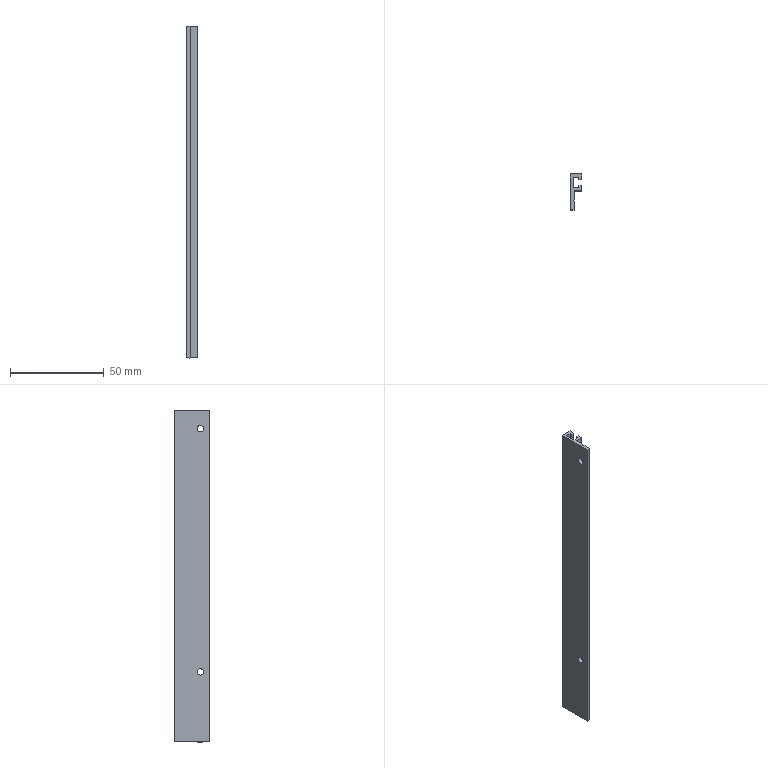Part | SolidWorks | features BaseBody 1 | 1 solid | 27 faces | box 6 x 19 x 177.5 mm | volume 9115 mm3 | plane 23 | cylinder 4 | commonest cylinder face diameters 3.4 x4
STEP:
#1=CARTESIAN_POINT('',(-62.496,1832.044,-25.2));
#2=VERTEX_POINT('',#1);
#3=CARTESIAN_POINT('',(-61.996,1831.544,-25.125));
#4=VERTEX_POINT('',#3);
#5=CARTESIAN_POINT('',(-62.496,1832.044,-25.2));
#6=CARTESIAN_POINT('',(-62.326,1831.874,-25.2));
#7=CARTESIAN_POINT('',(-62.158,1831.706,-25.175));
#8=CARTESIAN_POINT('',(-61.996,1831.544,-25.125));
#9=(BOUNDED_CURVE()B_SPLINE_CURVE(3,(#5,#6,#7,#8),.UNSPECIFIED.,.F.,.T.)B_SPLINE_CURVE_WITH_KNOTS((4,4),(1.571,1.869),.UNSPECIFIED.)CURVE()GEOMETRIC_REPRESENTATION_ITEM()RATIONAL_B_SPLINE_CURVE((1.,0.9926,0.9926,1.))REPRESENTATION_ITEM(''));
#10=EDGE_CURVE('',#2,#4,#9,.T.);
#11=ORIENTED_EDGE('',*,*,#10,.F.);
#12=CARTESIAN_POINT('',(-63.996,1832.044,-25.2));
#13=VERTEX_POINT('',#12);
#14=CARTESIAN_POINT('',(-63.996,1832.044,-25.2));
#15=DIRECTION('',(-1.,0.,0.));
#16=VECTOR('',#15,1000.);
#17=LINE('',#14,#16);
#18=EDGE_CURVE('',#2,#13,#17,.T.);
#19=ORIENTED_EDGE('',*,*,#18,.T.);
#20=CARTESIAN_POINT('',(-63.996,1832.044,-21.8));
#21=VERTEX_POINT('',#20);
#22=CARTESIAN_POINT('',(-63.996,1832.044,-23.5));
#23=DIRECTION('',(1.,0.,0.));
#24=DIRECTION('',(0.,0.,1.));
#25=AXIS2_PLACEMENT_3D('',#22,#23,#24);
#26=CIRCLE('',#25,1.7);
#27=EDGE_CURVE('',#21,#13,#26,.T.);
#28=ORIENTED_EDGE('',*,*,#27,.F.);
#29=CARTESIAN_POINT('',(-62.496,1832.044,-21.8));
#30=VERTEX_POINT('',#29);
#31=CARTESIAN_POINT('',(-63.996,1832.044,-21.8));
#32=DIRECTION('',(-1.,0.,0.));
#33=VECTOR('',#32,1000.);
#34=LINE('',#31,#33);
#35=EDGE_CURVE('',#30,#21,#34,.T.);
#36=ORIENTED_EDGE('',*,*,#35,.F.);
#37=CARTESIAN_POINT('',(-61.996,1831.544,-21.875));
#38=VERTEX_POINT('',#37);
#39=CARTESIAN_POINT('',(-61.996,1831.544,-21.875));
#40=CARTESIAN_POINT('',(-62.158,1831.706,-21.825));
#41=CARTESIAN_POINT('',(-62.326,1831.874,-21.8));
#42=CARTESIAN_POINT('',(-62.496,1832.044,-21.8));
#43=(BOUNDED_CURVE()B_SPLINE_CURVE(3,(#39,#40,#41,#42),.UNSPECIFIED.,.F.,.T.)B_SPLINE_CURVE_WITH_KNOTS((4,4),(4.414,4.712),.UNSPECIFIED.)CURVE()GEOMETRIC_REPRESENTATION_ITEM()RATIONAL_B_SPLINE_CURVE((1.,0.9926,0.9926,1.))REPRESENTATION_ITEM(''));
#44=EDGE_CURVE('',#38,#30,#43,.T.);
#45=ORIENTED_EDGE('',*,*,#44,.F.);
#46=CARTESIAN_POINT('',(-61.996,1832.044,-23.5));
#47=DIRECTION('',(-1.,0.,0.));
#48=DIRECTION('',(0.,0.,1.));
#49=AXIS2_PLACEMENT_3D('',#46,#47,#48);
#50=CIRCLE('',#49,1.7);
#51=EDGE_CURVE('',#4,#38,#50,.T.);
#52=ORIENTED_EDGE('',*,*,#51,.F.);
#53=EDGE_LOOP('',(#11,#19,#28,#36,#45,#52));
#54=FACE_OUTER_BOUND('',#53,.T.);
#55=CARTESIAN_POINT('',(-63.996,1832.044,-23.5));
#56=DIRECTION('',(-1.,0.,0.));
#57=DIRECTION('',(0.,0.,1.));
#58=AXIS2_PLACEMENT_3D('',#55,#56,#57);
#59=CYLINDRICAL_SURFACE('',#58,1.7);
#60=ADVANCED_FACE('',(#54),#59,.F.);
#61=CARTESIAN_POINT('',(-62.496,1832.044,-155.2));
#62=VERTEX_POINT('',#61);
#63=CARTESIAN_POINT('',(-61.996,1831.544,-155.125));
#64=VERTEX_POINT('',#63);
#65=CARTESIAN_POINT('',(-62.496,1832.044,-155.2));
#66=CARTESIAN_POINT('',(-62.326,1831.874,-155.2));
#67=CARTESIAN_POINT('',(-62.158,1831.706,-155.175));
#68=CARTESIAN_POINT('',(-61.996,1831.544,-155.125));
#69=(BOUNDED_CURVE()B_SPLINE_CURVE(3,(#65,#66,#67,#68),.UNSPECIFIED.,.F.,.T.)B_SPLINE_CURVE_WITH_KNOTS((4,4),(1.571,1.869),.UNSPECIFIED.)CURVE()GEOMETRIC_REPRESENTATION_ITEM()RATIONAL_B_SPLINE_CURVE((1.,0.9926,0.9926,1.))REPRESENTATION_ITEM(''));
#70=EDGE_CURVE('',#62,#64,#69,.T.);
#71=ORIENTED_EDGE('',*,*,#70,.F.);
#72=CARTESIAN_POINT('',(-63.996,1832.044,-155.2));
#73=VERTEX_POINT('',#72);
#74=CARTESIAN_POINT('',(-63.996,1832.044,-155.2));
#75=DIRECTION('',(-1.,0.,0.));
#76=VECTOR('',#75,1000.);
#77=LINE('',#74,#76);
#78=EDGE_CURVE('',#62,#73,#77,.T.);
#79=ORIENTED_EDGE('',*,*,#78,.T.);
#80=CARTESIAN_POINT('',(-63.996,1832.044,-151.8));
#81=VERTEX_POINT('',#80);
#82=CARTESIAN_POINT('',(-63.996,1832.044,-153.5));
#83=DIRECTION('',(1.,0.,0.));
#84=DIRECTION('',(0.,0.,1.));
#85=AXIS2_PLACEMENT_3D('',#82,#83,#84);
#86=CIRCLE('',#85,1.7);
#87=EDGE_CURVE('',#81,#73,#86,.T.);
#88=ORIENTED_EDGE('',*,*,#87,.F.);
#89=CARTESIAN_POINT('',(-62.496,1832.044,-151.8));
#90=VERTEX_POINT('',#89);
#91=CARTESIAN_POINT('',(-63.996,1832.044,-151.8));
#92=DIRECTION('',(-1.,0.,0.));
#93=VECTOR('',#92,1000.);
#94=LINE('',#91,#93);
#95=EDGE_CURVE('',#90,#81,#94,.T.);
#96=ORIENTED_EDGE('',*,*,#95,.F.);
#97=CARTESIAN_POINT('',(-61.996,1831.544,-151.875));
#98=VERTEX_POINT('',#97);
#99=CARTESIAN_POINT('',(-61.996,1831.544,-151.875));
#100=CARTESIAN_POINT('',(-62.158,1831.706,-151.825));
#101=CARTESIAN_POINT('',(-62.326,1831.874,-151.8));
#102=CARTESIAN_POINT('',(-62.496,1832.044,-151.8));
#103=(BOUNDED_CURVE()B_SPLINE_CURVE(3,(#99,#100,#101,#102),.UNSPECIFIED.,.F.,.T.)B_SPLINE_CURVE_WITH_KNOTS((4,4),(4.414,4.712),.UNSPECIFIED.)CURVE()GEOMETRIC_REPRESENTATION_ITEM()RATIONAL_B_SPLINE_CURVE((1.,0.9926,0.9926,1.))REPRESENTATION_ITEM(''));
#104=EDGE_CURVE('',#98,#90,#103,.T.);
#105=ORIENTED_EDGE('',*,*,#104,.F.);
#106=CARTESIAN_POINT('',(-61.996,1832.044,-153.5));
#107=DIRECTION('',(-1.,0.,0.));
#108=DIRECTION('',(0.,0.,1.));
#109=AXIS2_PLACEMENT_3D('',#106,#107,#108);
#110=CIRCLE('',#109,1.7);
#111=EDGE_CURVE('',#64,#98,#110,.T.);
#112=ORIENTED_EDGE('',*,*,#111,.F.);
#113=EDGE_LOOP('',(#71,#79,#88,#96,#105,#112));
#114=FACE_OUTER_BOUND('',#113,.T.);
#115=CARTESIAN_POINT('',(-63.996,1832.044,-153.5));
#116=DIRECTION('',(-1.,0.,0.));
#117=DIRECTION('',(0.,0.,1.));
#118=AXIS2_PLACEMENT_3D('',#115,#116,#117);
#119=CYLINDRICAL_SURFACE('',#118,1.7);
#120=ADVANCED_FACE('',(#114),#119,.F.);
#121=ORIENTED_EDGE('',*,*,#27,.T.);
#122=CARTESIAN_POINT('',(-63.996,1832.044,-23.5));
#123=DIRECTION('',(1.,0.,0.));
#124=DIRECTION('',(0.,0.,1.));
#125=AXIS2_PLACEMENT_3D('',#122,#123,#124);
#126=CIRCLE('',#125,1.7);
#127=EDGE_CURVE('',#13,#21,#126,.T.);
#128=ORIENTED_EDGE('',*,*,#127,.T.);
#129=EDGE_LOOP('',(#121,#128));
#130=FACE_BOUND('',#129,.T.);
#131=ORIENTED_EDGE('',*,*,#87,.T.);
#132=CARTESIAN_POINT('',(-63.996,1832.044,-153.5));
#133=DIRECTION('',(1.,0.,0.));
#134=DIRECTION('',(0.,0.,1.));
#135=AXIS2_PLACEMENT_3D('',#132,#133,#134);
#136=CIRCLE('',#135,1.7);
#137=EDGE_CURVE('',#73,#81,#136,.T.);
#138=ORIENTED_EDGE('',*,*,#137,.T.);
#139=EDGE_LOOP('',(#131,#138));
#140=FACE_BOUND('',#139,.T.);
#141=CARTESIAN_POINT('',(-63.996,1827.044,-191.));
#142=VERTEX_POINT('',#141);
#143=CARTESIAN_POINT('',(-63.996,1827.044,-13.5));
#144=VERTEX_POINT('',#143);
#145=CARTESIAN_POINT('',(-63.996,1827.044,206.5));
#146=DIRECTION('',(0.,0.,1.));
#147=VECTOR('',#146,1000.);
#148=LINE('',#145,#147);
#149=EDGE_CURVE('',#142,#144,#148,.T.);
#150=ORIENTED_EDGE('',*,*,#149,.T.);
#151=CARTESIAN_POINT('',(-63.996,1846.044,-13.5));
#152=VERTEX_POINT('',#151);
#153=CARTESIAN_POINT('',(-63.996,1846.044,-13.5));
#154=DIRECTION('',(0.,1.,0.));
#155=VECTOR('',#154,1000.);
#156=LINE('',#153,#155);
#157=EDGE_CURVE('',#144,#152,#156,.T.);
#158=ORIENTED_EDGE('',*,*,#157,.T.);
#159=CARTESIAN_POINT('',(-63.996,1846.044,-191.));
#160=VERTEX_POINT('',#159);
#161=CARTESIAN_POINT('',(-63.996,1846.044,206.5));
#162=DIRECTION('',(0.,0.,-1.));
#163=VECTOR('',#162,1000.);
#164=LINE('',#161,#163);
#165=EDGE_CURVE('',#152,#160,#164,.T.);
#166=ORIENTED_EDGE('',*,*,#165,.T.);
#167=CARTESIAN_POINT('',(-63.996,1846.044,-191.));
#168=DIRECTION('',(0.,-1.,0.));
#169=VECTOR('',#168,1000.);
#170=LINE('',#167,#169);
#171=EDGE_CURVE('',#160,#142,#170,.T.);
#172=ORIENTED_EDGE('',*,*,#171,.T.);
#173=EDGE_LOOP('',(#150,#158,#166,#172));
#174=FACE_OUTER_BOUND('',#173,.T.);
#175=CARTESIAN_POINT('',(-63.996,1846.044,206.5));
#176=DIRECTION('',(-1.,0.,0.));
#177=DIRECTION('',(0.,0.,1.));
#178=AXIS2_PLACEMENT_3D('',#175,#176,#177);
#179=PLANE('',#178);
#180=ADVANCED_FACE('',(#130,#140,#174),#179,.T.);
#181=ORIENTED_EDGE('',*,*,#18,.F.);
#182=CARTESIAN_POINT('',(-61.996,1832.544,-25.125));
#183=VERTEX_POINT('',#182);
#184=CARTESIAN_POINT('',(-61.996,1832.544,-25.125));
#185=CARTESIAN_POINT('',(-62.158,1832.382,-25.175));
#186=CARTESIAN_POINT('',(-62.326,1832.214,-25.2));
#187=CARTESIAN_POINT('',(-62.496,1832.044,-25.2));
#188=(BOUNDED_CURVE()B_SPLINE_CURVE(3,(#184,#185,#186,#187),.UNSPECIFIED.,.F.,.T.)B_SPLINE_CURVE_WITH_KNOTS((4,4),(4.414,4.712),.UNSPECIFIED.)CURVE()GEOMETRIC_REPRESENTATION_ITEM()RATIONAL_B_SPLINE_CURVE((1.,0.9926,0.9926,1.))REPRESENTATION_ITEM(''));
#189=EDGE_CURVE('',#183,#2,#188,.T.);
#190=ORIENTED_EDGE('',*,*,#189,.F.);
#191=CARTESIAN_POINT('',(-61.996,1832.544,-21.875));
#192=VERTEX_POINT('',#191);
#193=CARTESIAN_POINT('',(-61.996,1832.044,-23.5));
#194=DIRECTION('',(-1.,0.,0.));
#195=DIRECTION('',(0.,0.,1.));
#196=AXIS2_PLACEMENT_3D('',#193,#194,#195);
#197=CIRCLE('',#196,1.7);
#198=EDGE_CURVE('',#192,#183,#197,.T.);
#199=ORIENTED_EDGE('',*,*,#198,.F.);
#200=CARTESIAN_POINT('',(-62.496,1832.044,-21.8));
#201=CARTESIAN_POINT('',(-62.326,1832.214,-21.8));
#202=CARTESIAN_POINT('',(-62.158,1832.382,-21.825));
#203=CARTESIAN_POINT('',(-61.996,1832.544,-21.875));
#204=(BOUNDED_CURVE()B_SPLINE_CURVE(3,(#200,#201,#202,#203),.UNSPECIFIED.,.F.,.T.)B_SPLINE_CURVE_WITH_KNOTS((4,4),(1.571,1.869),.UNSPECIFIED.)CURVE()GEOMETRIC_REPRESENTATION_ITEM()RATIONAL_B_SPLINE_CURVE((1.,0.9926,0.9926,1.))REPRESENTATION_ITEM(''));
#205=EDGE_CURVE('',#30,#192,#204,.T.);
#206=ORIENTED_EDGE('',*,*,#205,.F.);
#207=ORIENTED_EDGE('',*,*,#35,.T.);
#208=ORIENTED_EDGE('',*,*,#127,.F.);
#209=EDGE_LOOP('',(#181,#190,#199,#206,#207,#208));
#210=FACE_OUTER_BOUND('',#209,.T.);
#211=CARTESIAN_POINT('',(-63.996,1832.044,-23.5));
#212=DIRECTION('',(-1.,0.,0.));
#213=DIRECTION('',(0.,0.,1.));
#214=AXIS2_PLACEMENT_3D('',#211,#212,#213);
#215=CYLINDRICAL_SURFACE('',#214,1.7);
#216=ADVANCED_FACE('',(#210),#215,.F.);
#217=ORIENTED_EDGE('',*,*,#78,.F.);
#218=CARTESIAN_POINT('',(-61.996,1832.544,-155.125));
#219=VERTEX_POINT('',#218);
#220=CARTESIAN_POINT('',(-61.996,1832.544,-155.125));
#221=CARTESIAN_POINT('',(-62.158,1832.382,-155.175));
#222=CARTESIAN_POINT('',(-62.326,1832.214,-155.2));
#223=CARTESIAN_POINT('',(-62.496,1832.044,-155.2));
#224=(BOUNDED_CURVE()B_SPLINE_CURVE(3,(#220,#221,#222,#223),.UNSPECIFIED.,.F.,.T.)B_SPLINE_CURVE_WITH_KNOTS((4,4),(4.414,4.712),.UNSPECIFIED.)CURVE()GEOMETRIC_REPRESENTATION_ITEM()RATIONAL_B_SPLINE_CURVE((1.,0.9926,0.9926,1.))REPRESENTATION_ITEM(''));
#225=EDGE_CURVE('',#219,#62,#224,.T.);
#226=ORIENTED_EDGE('',*,*,#225,.F.);
#227=CARTESIAN_POINT('',(-61.996,1832.544,-151.875));
#228=VERTEX_POINT('',#227);
#229=CARTESIAN_POINT('',(-61.996,1832.044,-153.5));
#230=DIRECTION('',(-1.,0.,0.));
#231=DIRECTION('',(0.,0.,1.));
#232=AXIS2_PLACEMENT_3D('',#229,#230,#231);
#233=CIRCLE('',#232,1.7);
#234=EDGE_CURVE('',#228,#219,#233,.T.);
#235=ORIENTED_EDGE('',*,*,#234,.F.);
#236=CARTESIAN_POINT('',(-62.496,1832.044,-151.8));
#237=CARTESIAN_POINT('',(-62.326,1832.214,-151.8));
#238=CARTESIAN_POINT('',(-62.158,1832.382,-151.825));
#239=CARTESIAN_POINT('',(-61.996,1832.544,-151.875));
#240=(BOUNDED_CURVE()B_SPLINE_CURVE(3,(#236,#237,#238,#239),.UNSPECIFIED.,.F.,.T.)B_SPLINE_CURVE_WITH_KNOTS((4,4),(1.571,1.869),.UNSPECIFIED.)CURVE()GEOMETRIC_REPRESENTATION_ITEM()RATIONAL_B_SPLINE_CURVE((1.,0.9926,0.9926,1.))REPRESENTATION_ITEM(''));
#241=EDGE_CURVE('',#90,#228,#240,.T.);
#242=ORIENTED_EDGE('',*,*,#241,.F.);
#243=ORIENTED_EDGE('',*,*,#95,.T.);
#244=ORIENTED_EDGE('',*,*,#137,.F.);
#245=EDGE_LOOP('',(#217,#226,#235,#242,#243,#244));
#246=FACE_OUTER_BOUND('',#245,.T.);
#247=CARTESIAN_POINT('',(-63.996,1832.044,-153.5));
#248=DIRECTION('',(-1.,0.,0.));
#249=DIRECTION('',(0.,0.,1.));
#250=AXIS2_PLACEMENT_3D('',#247,#248,#249);
#251=CYLINDRICAL_SURFACE('',#250,1.7);
#252=ADVANCED_FACE('',(#246),#251,.F.);
#253=CARTESIAN_POINT('',(-61.996,1827.044,-13.5));
#254=VERTEX_POINT('',#253);
#255=CARTESIAN_POINT('',(-63.996,1827.044,-13.5));
#256=DIRECTION('',(-1.,0.,0.));
#257=VECTOR('',#256,1000.);
#258=LINE('',#255,#257);
#259=EDGE_CURVE('',#254,#144,#258,.T.);
#260=ORIENTED_EDGE('',*,*,#259,.F.);
#261=CARTESIAN_POINT('',(-61.996,1831.544,-13.5));
#262=VERTEX_POINT('',#261);
#263=CARTESIAN_POINT('',(-61.996,1841.544,-13.5));
#264=DIRECTION('',(0.,-1.,0.));
#265=VECTOR('',#264,1000.);
#266=LINE('',#263,#265);
#267=EDGE_CURVE('',#262,#254,#266,.T.);
#268=ORIENTED_EDGE('',*,*,#267,.F.);
#269=CARTESIAN_POINT('',(-62.496,1832.044,-13.5));
#270=VERTEX_POINT('',#269);
#271=CARTESIAN_POINT('',(-62.496,1832.044,-13.5));
#272=DIRECTION('',(0.7071,-0.7071,0.));
#273=VECTOR('',#272,1000.);
#274=LINE('',#271,#273);
#275=EDGE_CURVE('',#270,#262,#274,.T.);
#276=ORIENTED_EDGE('',*,*,#275,.F.);
#277=CARTESIAN_POINT('',(-61.996,1832.544,-13.5));
#278=VERTEX_POINT('',#277);
#279=CARTESIAN_POINT('',(-61.996,1832.544,-13.5));
#280=DIRECTION('',(-0.7071,-0.7071,0.));
#281=VECTOR('',#280,1000.);
#282=LINE('',#279,#281);
#283=EDGE_CURVE('',#278,#270,#282,.T.);
#284=ORIENTED_EDGE('',*,*,#283,.F.);
#285=CARTESIAN_POINT('',(-61.996,1837.044,-13.5));
#286=VERTEX_POINT('',#285);
#287=CARTESIAN_POINT('',(-61.996,1841.544,-13.5));
#288=DIRECTION('',(0.,-1.,0.));
#289=VECTOR('',#288,1000.);
#290=LINE('',#287,#289);
#291=EDGE_CURVE('',#286,#278,#290,.T.);
#292=ORIENTED_EDGE('',*,*,#291,.F.);
#293=CARTESIAN_POINT('',(-57.996,1837.044,-13.5));
#294=VERTEX_POINT('',#293);
#295=CARTESIAN_POINT('',(-63.996,1837.044,-13.5));
#296=DIRECTION('',(-1.,0.,0.));
#297=VECTOR('',#296,1000.);
#298=LINE('',#295,#297);
#299=EDGE_CURVE('',#294,#286,#298,.T.);
#300=ORIENTED_EDGE('',*,*,#299,.F.);
#301=CARTESIAN_POINT('',(-57.996,1839.844,-13.5));
#302=VERTEX_POINT('',#301);
#303=CARTESIAN_POINT('',(-57.996,1841.544,-13.5));
#304=DIRECTION('',(0.,-1.,0.));
#305=VECTOR('',#304,1000.);
#306=LINE('',#303,#305);
#307=EDGE_CURVE('',#302,#294,#306,.T.);
#308=ORIENTED_EDGE('',*,*,#307,.F.);
#309=CARTESIAN_POINT('',(-59.496,1839.844,-13.5));
#310=VERTEX_POINT('',#309);
#311=CARTESIAN_POINT('',(-63.996,1839.844,-13.5));
#312=DIRECTION('',(1.,0.,0.));
#313=VECTOR('',#312,1000.);
#314=LINE('',#311,#313);
#315=EDGE_CURVE('',#310,#302,#314,.T.);
#316=ORIENTED_EDGE('',*,*,#315,.F.);
#317=CARTESIAN_POINT('',(-59.496,1838.694,-13.5));
#318=VERTEX_POINT('',#317);
#319=CARTESIAN_POINT('',(-59.496,1841.544,-13.5));
#320=DIRECTION('',(0.,1.,0.));
#321=VECTOR('',#320,1000.);
#322=LINE('',#319,#321);
#323=EDGE_CURVE('',#318,#310,#322,.T.);
#324=ORIENTED_EDGE('',*,*,#323,.F.);
#325=CARTESIAN_POINT('',(-62.496,1838.694,-13.5));
#326=VERTEX_POINT('',#325);
#327=CARTESIAN_POINT('',(-63.996,1838.694,-13.5));
#328=DIRECTION('',(1.,0.,0.));
#329=VECTOR('',#328,1000.);
#330=LINE('',#327,#329);
#331=EDGE_CURVE('',#326,#318,#330,.T.);
#332=ORIENTED_EDGE('',*,*,#331,.F.);
#333=CARTESIAN_POINT('',(-62.496,1844.394,-13.5));
#334=VERTEX_POINT('',#333);
#335=CARTESIAN_POINT('',(-62.496,1841.544,-13.5));
#336=DIRECTION('',(0.,-1.,0.));
#337=VECTOR('',#336,1000.);
#338=LINE('',#335,#337);
#339=EDGE_CURVE('',#334,#326,#338,.T.);
#340=ORIENTED_EDGE('',*,*,#339,.F.);
#341=CARTESIAN_POINT('',(-59.496,1844.394,-13.5));
#342=VERTEX_POINT('',#341);
#343=CARTESIAN_POINT('',(-63.996,1844.394,-13.5));
#344=DIRECTION('',(-1.,0.,0.));
#345=VECTOR('',#344,1000.);
#346=LINE('',#343,#345);
#347=EDGE_CURVE('',#342,#334,#346,.T.);
#348=ORIENTED_EDGE('',*,*,#347,.F.);
#349=CARTESIAN_POINT('',(-59.496,1843.244,-13.5));
#350=VERTEX_POINT('',#349);
#351=CARTESIAN_POINT('',(-59.496,1841.544,-13.5));
#352=DIRECTION('',(0.,1.,0.));
#353=VECTOR('',#352,1000.);
#354=LINE('',#351,#353);
#355=EDGE_CURVE('',#350,#342,#354,.T.);
#356=ORIENTED_EDGE('',*,*,#355,.F.);
#357=CARTESIAN_POINT('',(-57.996,1843.244,-13.5));
#358=VERTEX_POINT('',#357);
#359=CARTESIAN_POINT('',(-63.996,1843.244,-13.5));
#360=DIRECTION('',(-1.,0.,0.));
#361=VECTOR('',#360,1000.);
#362=LINE('',#359,#361);
#363=EDGE_CURVE('',#358,#350,#362,.T.);
#364=ORIENTED_EDGE('',*,*,#363,.F.);
#365=CARTESIAN_POINT('',(-57.996,1846.044,-13.5));
#366=VERTEX_POINT('',#365);
#367=CARTESIAN_POINT('',(-57.996,1841.544,-13.5));
#368=DIRECTION('',(0.,-1.,0.));
#369=VECTOR('',#368,1000.);
#370=LINE('',#367,#369);
#371=EDGE_CURVE('',#366,#358,#370,.T.);
#372=ORIENTED_EDGE('',*,*,#371,.F.);
#373=CARTESIAN_POINT('',(-63.996,1846.044,-13.5));
#374=DIRECTION('',(1.,0.,0.));
#375=VECTOR('',#374,1000.);
#376=LINE('',#373,#375);
#377=EDGE_CURVE('',#152,#366,#376,.T.);
#378=ORIENTED_EDGE('',*,*,#377,.F.);
#379=ORIENTED_EDGE('',*,*,#157,.F.);
#380=EDGE_LOOP('',(#260,#268,#276,#284,#292,#300,#308,#316,#324,#332,#340,#348,#356,#364,#372,#378,#379));
#381=FACE_OUTER_BOUND('',#380,.T.);
#382=CARTESIAN_POINT('',(-63.996,1841.544,-13.5));
#383=DIRECTION('',(0.,0.,-1.));
#384=DIRECTION('',(-1.,0.,0.));
#385=AXIS2_PLACEMENT_3D('',#382,#383,#384);
#386=PLANE('',#385);
#387=ADVANCED_FACE('',(#381),#386,.F.);
#388=CARTESIAN_POINT('',(-61.996,1827.044,-191.));
#389=VERTEX_POINT('',#388);
#390=CARTESIAN_POINT('',(-61.996,1827.044,206.5));
#391=DIRECTION('',(0.,0.,1.));
#392=VECTOR('',#391,1000.);
#393=LINE('',#390,#392);
#394=EDGE_CURVE('',#389,#254,#393,.T.);
#395=ORIENTED_EDGE('',*,*,#394,.T.);
#396=ORIENTED_EDGE('',*,*,#259,.T.);
#397=ORIENTED_EDGE('',*,*,#149,.F.);
#398=CARTESIAN_POINT('',(-63.996,1827.044,-191.));
#399=DIRECTION('',(1.,0.,0.));
#400=VECTOR('',#399,1000.);
#401=LINE('',#398,#400);
#402=EDGE_CURVE('',#142,#389,#401,.T.);
#403=ORIENTED_EDGE('',*,*,#402,.T.);
#404=EDGE_LOOP('',(#395,#396,#397,#403));
#405=FACE_OUTER_BOUND('',#404,.T.);
#406=CARTESIAN_POINT('',(-63.996,1827.044,206.5));
#407=DIRECTION('',(0.,-1.,0.));
#408=DIRECTION('',(0.,0.,-1.));
#409=AXIS2_PLACEMENT_3D('',#406,#407,#408);
#410=PLANE('',#409);
#411=ADVANCED_FACE('',(#405),#410,.T.);
#412=CARTESIAN_POINT('',(-61.996,1831.544,-191.));
#413=VERTEX_POINT('',#412);
#414=CARTESIAN_POINT('',(-61.996,1841.544,-191.));
#415=DIRECTION('',(0.,-1.,0.));
#416=VECTOR('',#415,1000.);
#417=LINE('',#414,#416);
#418=EDGE_CURVE('',#413,#389,#417,.T.);
#419=ORIENTED_EDGE('',*,*,#418,.T.);
#420=ORIENTED_EDGE('',*,*,#402,.F.);
#421=ORIENTED_EDGE('',*,*,#171,.F.);
#422=CARTESIAN_POINT('',(-57.996,1846.044,-191.));
#423=VERTEX_POINT('',#422);
#424=CARTESIAN_POINT('',(-63.996,1846.044,-191.));
#425=DIRECTION('',(1.,0.,0.));
#426=VECTOR('',#425,1000.);
#427=LINE('',#424,#426);
#428=EDGE_CURVE('',#160,#423,#427,.T.);
#429=ORIENTED_EDGE('',*,*,#428,.T.);
#430=CARTESIAN_POINT('',(-57.996,1843.244,-191.));
#431=VERTEX_POINT('',#430);
#432=CARTESIAN_POINT('',(-57.996,1841.544,-191.));
#433=DIRECTION('',(0.,-1.,0.));
#434=VECTOR('',#433,1000.);
#435=LINE('',#432,#434);
#436=EDGE_CURVE('',#423,#431,#435,.T.);
#437=ORIENTED_EDGE('',*,*,#436,.T.);
#438=CARTESIAN_POINT('',(-59.496,1843.244,-191.));
#439=VERTEX_POINT('',#438);
#440=CARTESIAN_POINT('',(-63.996,1843.244,-191.));
#441=DIRECTION('',(-1.,0.,0.));
#442=VECTOR('',#441,1000.);
#443=LINE('',#440,#442);
#444=EDGE_CURVE('',#431,#439,#443,.T.);
#445=ORIENTED_EDGE('',*,*,#444,.T.);
#446=CARTESIAN_POINT('',(-59.496,1844.394,-191.));
#447=VERTEX_POINT('',#446);
#448=CARTESIAN_POINT('',(-59.496,1841.544,-191.));
#449=DIRECTION('',(0.,1.,0.));
#450=VECTOR('',#449,1000.);
#451=LINE('',#448,#450);
#452=EDGE_CURVE('',#439,#447,#451,.T.);
#453=ORIENTED_EDGE('',*,*,#452,.T.);
#454=CARTESIAN_POINT('',(-62.496,1844.394,-191.));
#455=VERTEX_POINT('',#454);
#456=CARTESIAN_POINT('',(-63.996,1844.394,-191.));
#457=DIRECTION('',(-1.,0.,0.));
#458=VECTOR('',#457,1000.);
#459=LINE('',#456,#458);
#460=EDGE_CURVE('',#447,#455,#459,.T.);
#461=ORIENTED_EDGE('',*,*,#460,.T.);
#462=CARTESIAN_POINT('',(-62.496,1838.694,-191.));
#463=VERTEX_POINT('',#462);
#464=CARTESIAN_POINT('',(-62.496,1841.544,-191.));
#465=DIRECTION('',(0.,-1.,0.));
#466=VECTOR('',#465,1000.);
#467=LINE('',#464,#466);
#468=EDGE_CURVE('',#455,#463,#467,.T.);
#469=ORIENTED_EDGE('',*,*,#468,.T.);
#470=CARTESIAN_POINT('',(-59.496,1838.694,-191.));
#471=VERTEX_POINT('',#470);
#472=CARTESIAN_POINT('',(-63.996,1838.694,-191.));
#473=DIRECTION('',(1.,0.,0.));
#474=VECTOR('',#473,1000.);
#475=LINE('',#472,#474);
#476=EDGE_CURVE('',#463,#471,#475,.T.);
#477=ORIENTED_EDGE('',*,*,#476,.T.);
#478=CARTESIAN_POINT('',(-59.496,1839.844,-191.));
#479=VERTEX_POINT('',#478);
#480=CARTESIAN_POINT('',(-59.496,1841.544,-191.));
#481=DIRECTION('',(0.,1.,0.));
#482=VECTOR('',#481,1000.);
#483=LINE('',#480,#482);
#484=EDGE_CURVE('',#471,#479,#483,.T.);
#485=ORIENTED_EDGE('',*,*,#484,.T.);
#486=CARTESIAN_POINT('',(-57.996,1839.844,-191.));
#487=VERTEX_POINT('',#486);
#488=CARTESIAN_POINT('',(-63.996,1839.844,-191.));
#489=DIRECTION('',(1.,0.,0.));
#490=VECTOR('',#489,1000.);
#491=LINE('',#488,#490);
#492=EDGE_CURVE('',#479,#487,#491,.T.);
#493=ORIENTED_EDGE('',*,*,#492,.T.);
#494=CARTESIAN_POINT('',(-57.996,1837.044,-191.));
#495=VERTEX_POINT('',#494);
#496=CARTESIAN_POINT('',(-57.996,1841.544,-191.));
#497=DIRECTION('',(0.,-1.,0.));
#498=VECTOR('',#497,1000.);
#499=LINE('',#496,#498);
#500=EDGE_CURVE('',#487,#495,#499,.T.);
#501=ORIENTED_EDGE('',*,*,#500,.T.);
#502=CARTESIAN_POINT('',(-61.996,1837.044,-191.));
#503=VERTEX_POINT('',#502);
#504=CARTESIAN_POINT('',(-63.996,1837.044,-191.));
#505=DIRECTION('',(-1.,0.,0.));
#506=VECTOR('',#505,1000.);
#507=LINE('',#504,#506);
#508=EDGE_CURVE('',#495,#503,#507,.T.);
#509=ORIENTED_EDGE('',*,*,#508,.T.);
#510=CARTESIAN_POINT('',(-61.996,1832.544,-191.));
#511=VERTEX_POINT('',#510);
#512=CARTESIAN_POINT('',(-61.996,1841.544,-191.));
#513=DIRECTION('',(0.,-1.,0.));
#514=VECTOR('',#513,1000.);
#515=LINE('',#512,#514);
#516=EDGE_CURVE('',#503,#511,#515,.T.);
#517=ORIENTED_EDGE('',*,*,#516,.T.);
#518=CARTESIAN_POINT('',(-62.496,1832.044,-191.));
#519=VERTEX_POINT('',#518);
#520=CARTESIAN_POINT('',(-61.996,1832.544,-191.));
#521=DIRECTION('',(-0.7071,-0.7071,0.));
#522=VECTOR('',#521,1000.);
#523=LINE('',#520,#522);
#524=EDGE_CURVE('',#511,#519,#523,.T.);
#525=ORIENTED_EDGE('',*,*,#524,.T.);
#526=CARTESIAN_POINT('',(-62.496,1832.044,-191.));
#527=DIRECTION('',(0.7071,-0.7071,0.));
#528=VECTOR('',#527,1000.);
#529=LINE('',#526,#528);
#530=EDGE_CURVE('',#519,#413,#529,.T.);
#531=ORIENTED_EDGE('',*,*,#530,.T.);
#532=EDGE_LOOP('',(#419,#420,#421,#429,#437,#445,#453,#461,#469,#477,#485,#493,#501,#509,#517,#525,#531));
#533=FACE_OUTER_BOUND('',#532,.T.);
#534=CARTESIAN_POINT('',(-63.996,1841.544,-191.));
#535=DIRECTION('',(0.,0.,-1.));
#536=DIRECTION('',(-1.,0.,0.));
#537=AXIS2_PLACEMENT_3D('',#534,#535,#536);
#538=PLANE('',#537);
#539=ADVANCED_FACE('',(#533),#538,.T.);
#540=ORIENTED_EDGE('',*,*,#165,.F.);
#541=ORIENTED_EDGE('',*,*,#377,.T.);
#542=CARTESIAN_POINT('',(-57.996,1846.044,206.5));
#543=DIRECTION('',(0.,0.,-1.));
#544=VECTOR('',#543,1000.);
#545=LINE('',#542,#544);
#546=EDGE_CURVE('',#366,#423,#545,.T.);
#547=ORIENTED_EDGE('',*,*,#546,.T.);
#548=ORIENTED_EDGE('',*,*,#428,.F.);
#549=EDGE_LOOP('',(#540,#541,#547,#548));
#550=FACE_OUTER_BOUND('',#549,.T.);
#551=CARTESIAN_POINT('',(-57.996,1846.044,206.5));
#552=DIRECTION('',(0.,1.,0.));
#553=DIRECTION('',(0.,0.,1.));
#554=AXIS2_PLACEMENT_3D('',#551,#552,#553);
#555=PLANE('',#554);
#556=ADVANCED_FACE('',(#550),#555,.T.);
#557=CARTESIAN_POINT('',(-62.496,1832.044,-13.5));
#558=DIRECTION('',(0.,0.,-1.));
#559=VECTOR('',#558,1000.);
#560=LINE('',#557,#559);
#561=EDGE_CURVE('',#270,#30,#560,.T.);
#562=ORIENTED_EDGE('',*,*,#561,.T.);
#563=ORIENTED_EDGE('',*,*,#205,.T.);
#564=CARTESIAN_POINT('',(-61.996,1832.544,-13.5));
#565=DIRECTION('',(0.,0.,1.));
#566=VECTOR('',#565,1000.);
#567=LINE('',#564,#566);
#568=EDGE_CURVE('',#192,#278,#567,.T.);
#569=ORIENTED_EDGE('',*,*,#568,.T.);
#570=ORIENTED_EDGE('',*,*,#283,.T.);
#571=EDGE_LOOP('',(#562,#563,#569,#570));
#572=FACE_OUTER_BOUND('',#571,.T.);
#573=CARTESIAN_POINT('',(-62.496,1832.044,-13.5));
#574=DIRECTION('',(0.7071,-0.7071,0.));
#575=DIRECTION('',(0.7071,0.7071,0.));
#576=AXIS2_PLACEMENT_3D('',#573,#574,#575);
#577=PLANE('',#576);
#578=ADVANCED_FACE('',(#572),#577,.T.);
#579=CARTESIAN_POINT('',(-61.996,1831.544,-13.5));
#580=DIRECTION('',(0.,0.,-1.));
#581=VECTOR('',#580,1000.);
#582=LINE('',#579,#581);
#583=EDGE_CURVE('',#262,#38,#582,.T.);
#584=ORIENTED_EDGE('',*,*,#583,.T.);
#585=ORIENTED_EDGE('',*,*,#44,.T.);
#586=ORIENTED_EDGE('',*,*,#561,.F.);
#587=ORIENTED_EDGE('',*,*,#275,.T.);
#588=EDGE_LOOP('',(#584,#585,#586,#587));
#589=FACE_OUTER_BOUND('',#588,.T.);
#590=CARTESIAN_POINT('',(-61.996,1831.544,-13.5));
#591=DIRECTION('',(0.7071,0.7071,0.));
#592=DIRECTION('',(-0.7071,0.7071,0.));
#593=AXIS2_PLACEMENT_3D('',#590,#591,#592);
#594=PLANE('',#593);
#595=ADVANCED_FACE('',(#589),#594,.T.);
#596=CARTESIAN_POINT('',(-61.996,1831.544,206.5));
#597=DIRECTION('',(0.,0.,1.));
#598=VECTOR('',#597,1000.);
#599=LINE('',#596,#598);
#600=EDGE_CURVE('',#413,#64,#599,.T.);
#601=ORIENTED_EDGE('',*,*,#600,.T.);
#602=ORIENTED_EDGE('',*,*,#111,.T.);
#603=CARTESIAN_POINT('',(-61.996,1831.544,206.5));
#604=DIRECTION('',(0.,0.,1.));
#605=VECTOR('',#604,1000.);
#606=LINE('',#603,#605);
#607=EDGE_CURVE('',#98,#4,#606,.T.);
#608=ORIENTED_EDGE('',*,*,#607,.T.);
#609=ORIENTED_EDGE('',*,*,#51,.T.);
#610=ORIENTED_EDGE('',*,*,#583,.F.);
#611=ORIENTED_EDGE('',*,*,#267,.T.);
#612=ORIENTED_EDGE('',*,*,#394,.F.);
#613=ORIENTED_EDGE('',*,*,#418,.F.);
#614=EDGE_LOOP('',(#601,#602,#608,#609,#610,#611,#612,#613));
#615=FACE_OUTER_BOUND('',#614,.T.);
#616=CARTESIAN_POINT('',(-61.996,1827.044,206.5));
#617=DIRECTION('',(1.,0.,0.));
#618=DIRECTION('',(0.,0.,-1.));
#619=AXIS2_PLACEMENT_3D('',#616,#617,#618);
#620=PLANE('',#619);
#621=ADVANCED_FACE('',(#615),#620,.T.);
#622=ORIENTED_EDGE('',*,*,#568,.F.);
#623=ORIENTED_EDGE('',*,*,#198,.T.);
#624=CARTESIAN_POINT('',(-61.996,1832.544,206.5));
#625=DIRECTION('',(0.,0.,-1.));
#626=VECTOR('',#625,1000.);
#627=LINE('',#624,#626);
#628=EDGE_CURVE('',#183,#228,#627,.T.);
#629=ORIENTED_EDGE('',*,*,#628,.T.);
#630=ORIENTED_EDGE('',*,*,#234,.T.);
#631=CARTESIAN_POINT('',(-61.996,1832.544,206.5));
#632=DIRECTION('',(0.,0.,-1.));
#633=VECTOR('',#632,1000.);
#634=LINE('',#631,#633);
#635=EDGE_CURVE('',#219,#511,#634,.T.);
#636=ORIENTED_EDGE('',*,*,#635,.T.);
#637=ORIENTED_EDGE('',*,*,#516,.F.);
#638=CARTESIAN_POINT('',(-61.996,1837.044,206.5));
#639=DIRECTION('',(0.,0.,1.));
#640=VECTOR('',#639,1000.);
#641=LINE('',#638,#640);
#642=EDGE_CURVE('',#503,#286,#641,.T.);
#643=ORIENTED_EDGE('',*,*,#642,.T.);
#644=ORIENTED_EDGE('',*,*,#291,.T.);
#645=EDGE_LOOP('',(#622,#623,#629,#630,#636,#637,#643,#644));
#646=FACE_OUTER_BOUND('',#645,.T.);
#647=CARTESIAN_POINT('',(-61.996,1832.544,206.5));
#648=DIRECTION('',(1.,0.,0.));
#649=DIRECTION('',(0.,0.,-1.));
#650=AXIS2_PLACEMENT_3D('',#647,#648,#649);
#651=PLANE('',#650);
#652=ADVANCED_FACE('',(#646),#651,.T.);
#653=ORIENTED_EDGE('',*,*,#628,.F.);
#654=ORIENTED_EDGE('',*,*,#189,.T.);
#655=CARTESIAN_POINT('',(-62.496,1832.044,-13.5));
#656=DIRECTION('',(0.,0.,-1.));
#657=VECTOR('',#656,1000.);
#658=LINE('',#655,#657);
#659=EDGE_CURVE('',#2,#90,#658,.T.);
#660=ORIENTED_EDGE('',*,*,#659,.T.);
#661=ORIENTED_EDGE('',*,*,#241,.T.);
#662=EDGE_LOOP('',(#653,#654,#660,#661));
#663=FACE_OUTER_BOUND('',#662,.T.);
#664=CARTESIAN_POINT('',(-62.496,1832.044,-13.5));
#665=DIRECTION('',(0.7071,-0.7071,0.));
#666=DIRECTION('',(0.7071,0.7071,0.));
#667=AXIS2_PLACEMENT_3D('',#664,#665,#666);
#668=PLANE('',#667);
#669=ADVANCED_FACE('',(#663),#668,.T.);
#670=ORIENTED_EDGE('',*,*,#659,.F.);
#671=ORIENTED_EDGE('',*,*,#10,.T.);
#672=ORIENTED_EDGE('',*,*,#607,.F.);
#673=ORIENTED_EDGE('',*,*,#104,.T.);
#674=EDGE_LOOP('',(#670,#671,#672,#673));
#675=FACE_OUTER_BOUND('',#674,.T.);
#676=CARTESIAN_POINT('',(-61.996,1831.544,-13.5));
#677=DIRECTION('',(0.7071,0.7071,0.));
#678=DIRECTION('',(-0.7071,0.7071,0.));
#679=AXIS2_PLACEMENT_3D('',#676,#677,#678);
#680=PLANE('',#679);
#681=ADVANCED_FACE('',(#675),#680,.T.);
#682=ORIENTED_EDGE('',*,*,#635,.F.);
#683=ORIENTED_EDGE('',*,*,#225,.T.);
#684=CARTESIAN_POINT('',(-62.496,1832.044,206.5));
#685=DIRECTION('',(0.,0.,-1.));
#686=VECTOR('',#685,1000.);
#687=LINE('',#684,#686);
#688=EDGE_CURVE('',#62,#519,#687,.T.);
#689=ORIENTED_EDGE('',*,*,#688,.T.);
#690=ORIENTED_EDGE('',*,*,#524,.F.);
#691=EDGE_LOOP('',(#682,#683,#689,#690));
#692=FACE_OUTER_BOUND('',#691,.T.);
#693=CARTESIAN_POINT('',(-62.496,1832.044,206.5));
#694=DIRECTION('',(0.7071,-0.7071,0.));
#695=DIRECTION('',(0.7071,0.7071,0.));
#696=AXIS2_PLACEMENT_3D('',#693,#694,#695);
#697=PLANE('',#696);
#698=ADVANCED_FACE('',(#692),#697,.T.);
#699=ORIENTED_EDGE('',*,*,#688,.F.);
#700=ORIENTED_EDGE('',*,*,#70,.T.);
#701=ORIENTED_EDGE('',*,*,#600,.F.);
#702=ORIENTED_EDGE('',*,*,#530,.F.);
#703=EDGE_LOOP('',(#699,#700,#701,#702));
#704=FACE_OUTER_BOUND('',#703,.T.);
#705=CARTESIAN_POINT('',(-61.996,1831.544,206.5));
#706=DIRECTION('',(0.7071,0.7071,0.));
#707=DIRECTION('',(-0.7071,0.7071,0.));
#708=AXIS2_PLACEMENT_3D('',#705,#706,#707);
#709=PLANE('',#708);
#710=ADVANCED_FACE('',(#704),#709,.T.);
#711=CARTESIAN_POINT('',(-57.996,1837.044,206.5));
#712=DIRECTION('',(0.,0.,1.));
#713=VECTOR('',#712,1000.);
#714=LINE('',#711,#713);
#715=EDGE_CURVE('',#495,#294,#714,.T.);
#716=ORIENTED_EDGE('',*,*,#715,.T.);
#717=ORIENTED_EDGE('',*,*,#299,.T.);
#718=ORIENTED_EDGE('',*,*,#642,.F.);
#719=ORIENTED_EDGE('',*,*,#508,.F.);
#720=EDGE_LOOP('',(#716,#717,#718,#719));
#721=FACE_OUTER_BOUND('',#720,.T.);
#722=CARTESIAN_POINT('',(-61.996,1837.044,206.5));
#723=DIRECTION('',(0.,-1.,0.));
#724=DIRECTION('',(0.,0.,-1.));
#725=AXIS2_PLACEMENT_3D('',#722,#723,#724);
#726=PLANE('',#725);
#727=ADVANCED_FACE('',(#721),#726,.T.);
#728=CARTESIAN_POINT('',(-57.996,1839.844,206.5));
#729=DIRECTION('',(0.,0.,1.));
#730=VECTOR('',#729,1000.);
#731=LINE('',#728,#730);
#732=EDGE_CURVE('',#487,#302,#731,.T.);
#733=ORIENTED_EDGE('',*,*,#732,.T.);
#734=ORIENTED_EDGE('',*,*,#307,.T.);
#735=ORIENTED_EDGE('',*,*,#715,.F.);
#736=ORIENTED_EDGE('',*,*,#500,.F.);
#737=EDGE_LOOP('',(#733,#734,#735,#736));
#738=FACE_OUTER_BOUND('',#737,.T.);
#739=CARTESIAN_POINT('',(-57.996,1837.044,206.5));
#740=DIRECTION('',(1.,0.,0.));
#741=DIRECTION('',(0.,0.,-1.));
#742=AXIS2_PLACEMENT_3D('',#739,#740,#741);
#743=PLANE('',#742);
#744=ADVANCED_FACE('',(#738),#743,.T.);
#745=CARTESIAN_POINT('',(-59.496,1839.844,206.5));
#746=DIRECTION('',(0.,0.,1.));
#747=VECTOR('',#746,1000.);
#748=LINE('',#745,#747);
#749=EDGE_CURVE('',#479,#310,#748,.T.);
#750=ORIENTED_EDGE('',*,*,#749,.T.);
#751=ORIENTED_EDGE('',*,*,#315,.T.);
#752=ORIENTED_EDGE('',*,*,#732,.F.);
#753=ORIENTED_EDGE('',*,*,#492,.F.);
#754=EDGE_LOOP('',(#750,#751,#752,#753));
#755=FACE_OUTER_BOUND('',#754,.T.);
#756=CARTESIAN_POINT('',(-57.996,1839.844,206.5));
#757=DIRECTION('',(0.,1.,0.));
#758=DIRECTION('',(0.,0.,1.));
#759=AXIS2_PLACEMENT_3D('',#756,#757,#758);
#760=PLANE('',#759);
#761=ADVANCED_FACE('',(#755),#760,.T.);
#762=CARTESIAN_POINT('',(-59.496,1838.694,206.5));
#763=DIRECTION('',(0.,0.,1.));
#764=VECTOR('',#763,1000.);
#765=LINE('',#762,#764);
#766=EDGE_CURVE('',#471,#318,#765,.T.);
#767=ORIENTED_EDGE('',*,*,#766,.T.);
#768=ORIENTED_EDGE('',*,*,#323,.T.);
#769=ORIENTED_EDGE('',*,*,#749,.F.);
#770=ORIENTED_EDGE('',*,*,#484,.F.);
#771=EDGE_LOOP('',(#767,#768,#769,#770));
#772=FACE_OUTER_BOUND('',#771,.T.);
#773=CARTESIAN_POINT('',(-59.496,1839.844,206.5));
#774=DIRECTION('',(-1.,0.,0.));
#775=DIRECTION('',(0.,0.,1.));
#776=AXIS2_PLACEMENT_3D('',#773,#774,#775);
#777=PLANE('',#776);
#778=ADVANCED_FACE('',(#772),#777,.T.);
#779=CARTESIAN_POINT('',(-62.496,1838.694,206.5));
#780=DIRECTION('',(0.,0.,1.));
#781=VECTOR('',#780,1000.);
#782=LINE('',#779,#781);
#783=EDGE_CURVE('',#463,#326,#782,.T.);
#784=ORIENTED_EDGE('',*,*,#783,.T.);
#785=ORIENTED_EDGE('',*,*,#331,.T.);
#786=ORIENTED_EDGE('',*,*,#766,.F.);
#787=ORIENTED_EDGE('',*,*,#476,.F.);
#788=EDGE_LOOP('',(#784,#785,#786,#787));
#789=FACE_OUTER_BOUND('',#788,.T.);
#790=CARTESIAN_POINT('',(-59.496,1838.694,206.5));
#791=DIRECTION('',(0.,1.,0.));
#792=DIRECTION('',(0.,0.,1.));
#793=AXIS2_PLACEMENT_3D('',#790,#791,#792);
#794=PLANE('',#793);
#795=ADVANCED_FACE('',(#789),#794,.T.);
#796=CARTESIAN_POINT('',(-62.496,1844.394,206.5));
#797=DIRECTION('',(0.,0.,1.));
#798=VECTOR('',#797,1000.);
#799=LINE('',#796,#798);
#800=EDGE_CURVE('',#455,#334,#799,.T.);
#801=ORIENTED_EDGE('',*,*,#800,.T.);
#802=ORIENTED_EDGE('',*,*,#339,.T.);
#803=ORIENTED_EDGE('',*,*,#783,.F.);
#804=ORIENTED_EDGE('',*,*,#468,.F.);
#805=EDGE_LOOP('',(#801,#802,#803,#804));
#806=FACE_OUTER_BOUND('',#805,.T.);
#807=CARTESIAN_POINT('',(-62.496,1838.694,206.5));
#808=DIRECTION('',(1.,0.,0.));
#809=DIRECTION('',(0.,0.,-1.));
#810=AXIS2_PLACEMENT_3D('',#807,#808,#809);
#811=PLANE('',#810);
#812=ADVANCED_FACE('',(#806),#811,.T.);
#813=CARTESIAN_POINT('',(-59.496,1844.394,206.5));
#814=DIRECTION('',(0.,0.,1.));
#815=VECTOR('',#814,1000.);
#816=LINE('',#813,#815);
#817=EDGE_CURVE('',#447,#342,#816,.T.);
#818=ORIENTED_EDGE('',*,*,#817,.T.);
#819=ORIENTED_EDGE('',*,*,#347,.T.);
#820=ORIENTED_EDGE('',*,*,#800,.F.);
#821=ORIENTED_EDGE('',*,*,#460,.F.);
#822=EDGE_LOOP('',(#818,#819,#820,#821));
#823=FACE_OUTER_BOUND('',#822,.T.);
#824=CARTESIAN_POINT('',(-62.496,1844.394,206.5));
#825=DIRECTION('',(0.,-1.,0.));
#826=DIRECTION('',(0.,0.,-1.));
#827=AXIS2_PLACEMENT_3D('',#824,#825,#826);
#828=PLANE('',#827);
#829=ADVANCED_FACE('',(#823),#828,.T.);
#830=CARTESIAN_POINT('',(-59.496,1843.244,206.5));
#831=DIRECTION('',(0.,0.,1.));
#832=VECTOR('',#831,1000.);
#833=LINE('',#830,#832);
#834=EDGE_CURVE('',#439,#350,#833,.T.);
#835=ORIENTED_EDGE('',*,*,#834,.T.);
#836=ORIENTED_EDGE('',*,*,#355,.T.);
#837=ORIENTED_EDGE('',*,*,#817,.F.);
#838=ORIENTED_EDGE('',*,*,#452,.F.);
#839=EDGE_LOOP('',(#835,#836,#837,#838));
#840=FACE_OUTER_BOUND('',#839,.T.);
#841=CARTESIAN_POINT('',(-59.496,1844.394,206.5));
#842=DIRECTION('',(-1.,0.,0.));
#843=DIRECTION('',(0.,0.,1.));
#844=AXIS2_PLACEMENT_3D('',#841,#842,#843);
#845=PLANE('',#844);
#846=ADVANCED_FACE('',(#840),#845,.T.);
#847=CARTESIAN_POINT('',(-57.996,1843.244,206.5));
#848=DIRECTION('',(0.,0.,1.));
#849=VECTOR('',#848,1000.);
#850=LINE('',#847,#849);
#851=EDGE_CURVE('',#431,#358,#850,.T.);
#852=ORIENTED_EDGE('',*,*,#851,.T.);
#853=ORIENTED_EDGE('',*,*,#363,.T.);
#854=ORIENTED_EDGE('',*,*,#834,.F.);
#855=ORIENTED_EDGE('',*,*,#444,.F.);
#856=EDGE_LOOP('',(#852,#853,#854,#855));
#857=FACE_OUTER_BOUND('',#856,.T.);
#858=CARTESIAN_POINT('',(-59.496,1843.244,206.5));
#859=DIRECTION('',(0.,-1.,0.));
#860=DIRECTION('',(0.,0.,-1.));
#861=AXIS2_PLACEMENT_3D('',#858,#859,#860);
#862=PLANE('',#861);
#863=ADVANCED_FACE('',(#857),#862,.T.);
#864=ORIENTED_EDGE('',*,*,#546,.F.);
#865=ORIENTED_EDGE('',*,*,#371,.T.);
#866=ORIENTED_EDGE('',*,*,#851,.F.);
#867=ORIENTED_EDGE('',*,*,#436,.F.);
#868=EDGE_LOOP('',(#864,#865,#866,#867));
#869=FACE_OUTER_BOUND('',#868,.T.);
#870=CARTESIAN_POINT('',(-57.996,1843.244,206.5));
#871=DIRECTION('',(1.,0.,0.));
#872=DIRECTION('',(0.,0.,-1.));
#873=AXIS2_PLACEMENT_3D('',#870,#871,#872);
#874=PLANE('',#873);
#875=ADVANCED_FACE('',(#869),#874,.T.);
#876=CLOSED_SHELL('',(#60,#120,#180,#216,#252,#387,#411,#539,#556,#578,#595,#621,#652,#669,#681,#698,#710,#727,#744,#761,#778,#795,#812,#829,#846,#863,#875));
#877=MANIFOLD_SOLID_BREP('',#876);
#878=CARTESIAN_POINT('',(0.,0.,0.));
#879=DIRECTION('',(0.,0.,1.));
#880=DIRECTION('',(1.,0.,0.));
#881=AXIS2_PLACEMENT_3D('',#878,#879,#880);
#882=(LENGTH_UNIT()NAMED_UNIT(*)SI_UNIT(.MILLI.,.METRE.));
#883=UNCERTAINTY_MEASURE_WITH_UNIT(LENGTH_MEASURE(0.00001),#882,'','');
#884=(NAMED_UNIT(*)PLANE_ANGLE_UNIT()SI_UNIT($,.RADIAN.));
#885=(NAMED_UNIT(*)SI_UNIT($,.STERADIAN.)SOLID_ANGLE_UNIT());
#886=(GEOMETRIC_REPRESENTATION_CONTEXT(3)GLOBAL_UNCERTAINTY_ASSIGNED_CONTEXT((#883))GLOBAL_UNIT_ASSIGNED_CONTEXT((#882,#884,#885))REPRESENTATION_CONTEXT('',''));
#887=ADVANCED_BREP_SHAPE_REPRESENTATION('',(#877,#881),#886);